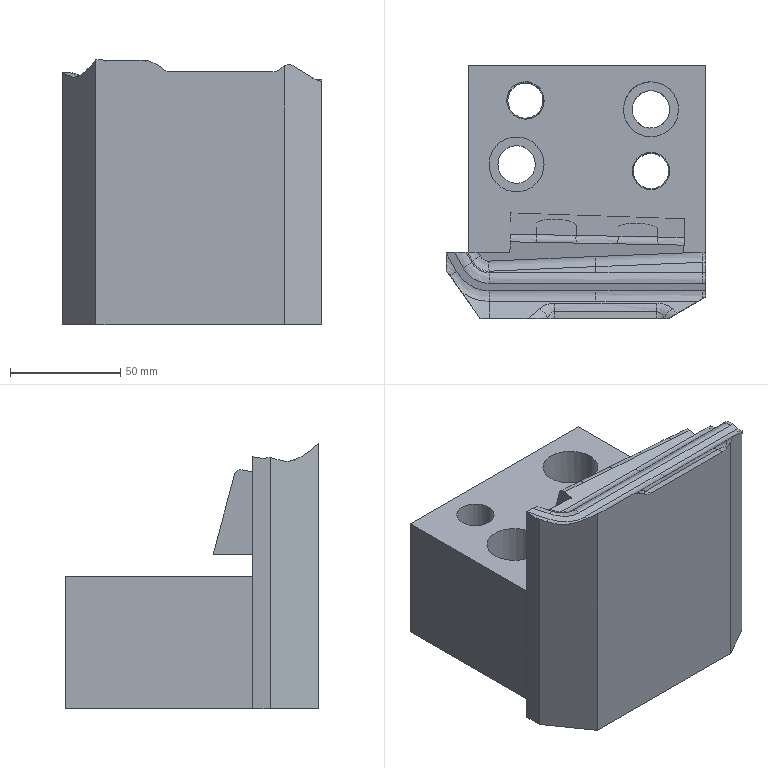Part | NX | features solid 2 | 1 solid | 67 faces | box 117.926 x 115 x 120.411 mm | volume 877573 mm3 | spline 40 | plane 19 | cylinder 8 | commonest cylinder face diameters 17 x4 16 x2 25 x2